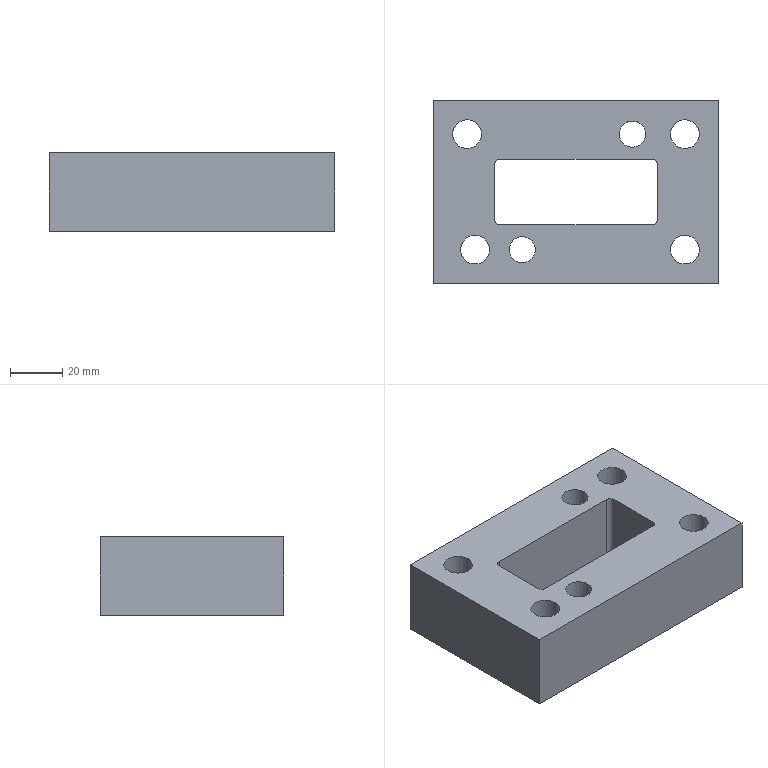Part | STEP file | 213_id694_x_t | 1 solid | 32 faces | box 109 x 70 x 30 mm | volume 157975 mm3 | plane 16 | cylinder 16 | commonest cylinder face diameters 11 x6 4 x4 17 x4 10 x2